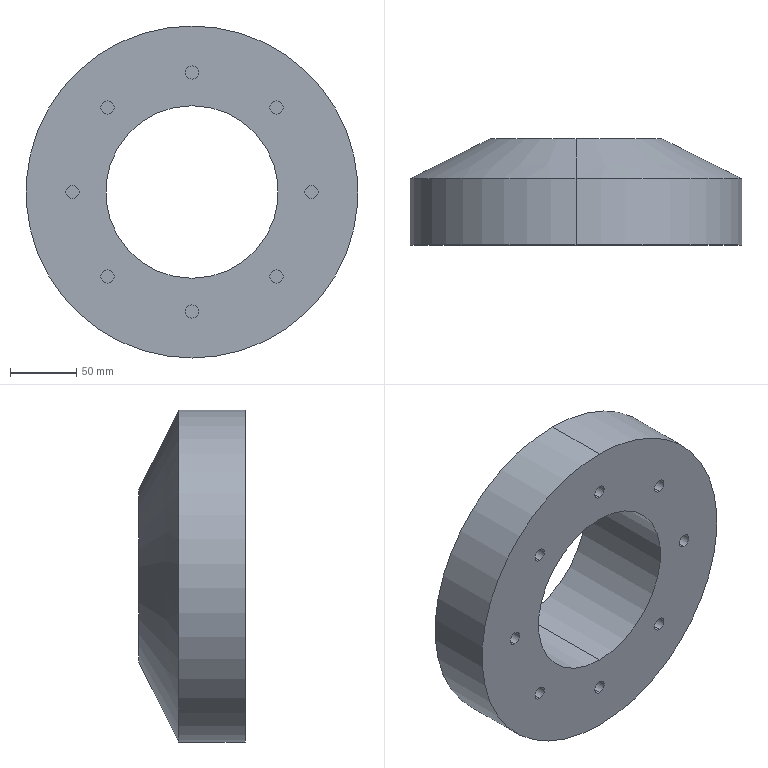Part | SolidWorks | features ICE 1, Revolution 1 | 1 solid | 31 faces | box 250 x 80 x 250 mm | volume 2252522 mm3 | cylinder 20 | plane 9 | cone 2 | commonest cylinder face diameters 10 x16 130 x2 250 x2
STEP:
#1=CARTESIAN_POINT('',(63.64,-23.992,-58.64));
#2=VERTEX_POINT('',#1);
#3=CARTESIAN_POINT('',(63.64,-23.992,-68.64));
#4=VERTEX_POINT('',#3);
#5=CARTESIAN_POINT('',(63.64,-23.992,-63.64));
#6=DIRECTION('',(0.,-1.,0.));
#7=DIRECTION('',(0.,0.,-1.));
#8=AXIS2_PLACEMENT_3D('',#5,#6,#7);
#9=CIRCLE('',#8,5.);
#10=EDGE_CURVE('',#2,#4,#9,.T.);
#11=ORIENTED_EDGE('',*,*,#10,.F.);
#12=CARTESIAN_POINT('',(63.64,-53.992,-58.64));
#13=VERTEX_POINT('',#12);
#14=CARTESIAN_POINT('',(63.64,-23.992,-58.64));
#15=DIRECTION('',(0.,-1.,0.));
#16=VECTOR('',#15,1000.);
#17=LINE('',#14,#16);
#18=EDGE_CURVE('',#2,#13,#17,.T.);
#19=ORIENTED_EDGE('',*,*,#18,.T.);
#20=CARTESIAN_POINT('',(63.64,-53.992,-68.64));
#21=VERTEX_POINT('',#20);
#22=CARTESIAN_POINT('',(63.64,-53.992,-63.64));
#23=DIRECTION('',(0.,-1.,0.));
#24=DIRECTION('',(0.,0.,-1.));
#25=AXIS2_PLACEMENT_3D('',#22,#23,#24);
#26=CIRCLE('',#25,5.);
#27=EDGE_CURVE('',#13,#21,#26,.T.);
#28=ORIENTED_EDGE('',*,*,#27,.T.);
#29=CARTESIAN_POINT('',(63.64,-23.992,-68.64));
#30=DIRECTION('',(0.,-1.,0.));
#31=VECTOR('',#30,1000.);
#32=LINE('',#29,#31);
#33=EDGE_CURVE('',#4,#21,#32,.T.);
#34=ORIENTED_EDGE('',*,*,#33,.F.);
#35=EDGE_LOOP('',(#11,#19,#28,#34));
#36=FACE_OUTER_BOUND('',#35,.T.);
#37=CARTESIAN_POINT('',(63.64,-23.992,-63.64));
#38=DIRECTION('',(0.,-1.,0.));
#39=DIRECTION('',(0.,0.,-1.));
#40=AXIS2_PLACEMENT_3D('',#37,#38,#39);
#41=CYLINDRICAL_SURFACE('',#40,5.);
#42=ADVANCED_FACE('',(#36),#41,.F.);
#43=CARTESIAN_POINT('',(0.,-23.992,-85.));
#44=VERTEX_POINT('',#43);
#45=CARTESIAN_POINT('',(0.,-23.992,-95.));
#46=VERTEX_POINT('',#45);
#47=CARTESIAN_POINT('',(0.,-23.992,-90.));
#48=DIRECTION('',(0.,-1.,0.));
#49=DIRECTION('',(0.,0.,-1.));
#50=AXIS2_PLACEMENT_3D('',#47,#48,#49);
#51=CIRCLE('',#50,5.);
#52=EDGE_CURVE('',#44,#46,#51,.T.);
#53=ORIENTED_EDGE('',*,*,#52,.F.);
#54=CARTESIAN_POINT('',(0.,-53.992,-85.));
#55=VERTEX_POINT('',#54);
#56=CARTESIAN_POINT('',(0.,-23.992,-85.));
#57=DIRECTION('',(0.,-1.,0.));
#58=VECTOR('',#57,1000.);
#59=LINE('',#56,#58);
#60=EDGE_CURVE('',#44,#55,#59,.T.);
#61=ORIENTED_EDGE('',*,*,#60,.T.);
#62=CARTESIAN_POINT('',(0.,-53.992,-95.));
#63=VERTEX_POINT('',#62);
#64=CARTESIAN_POINT('',(0.,-53.992,-90.));
#65=DIRECTION('',(0.,-1.,0.));
#66=DIRECTION('',(0.,0.,-1.));
#67=AXIS2_PLACEMENT_3D('',#64,#65,#66);
#68=CIRCLE('',#67,5.);
#69=EDGE_CURVE('',#55,#63,#68,.T.);
#70=ORIENTED_EDGE('',*,*,#69,.T.);
#71=CARTESIAN_POINT('',(0.,-23.992,-95.));
#72=DIRECTION('',(0.,-1.,0.));
#73=VECTOR('',#72,1000.);
#74=LINE('',#71,#73);
#75=EDGE_CURVE('',#46,#63,#74,.T.);
#76=ORIENTED_EDGE('',*,*,#75,.F.);
#77=EDGE_LOOP('',(#53,#61,#70,#76));
#78=FACE_OUTER_BOUND('',#77,.T.);
#79=CARTESIAN_POINT('',(0.,-23.992,-90.));
#80=DIRECTION('',(0.,-1.,0.));
#81=DIRECTION('',(0.,0.,-1.));
#82=AXIS2_PLACEMENT_3D('',#79,#80,#81);
#83=CYLINDRICAL_SURFACE('',#82,5.);
#84=ADVANCED_FACE('',(#78),#83,.F.);
#85=CARTESIAN_POINT('',(-63.64,-23.992,-58.64));
#86=VERTEX_POINT('',#85);
#87=CARTESIAN_POINT('',(-63.64,-23.992,-68.64));
#88=VERTEX_POINT('',#87);
#89=CARTESIAN_POINT('',(-63.64,-23.992,-63.64));
#90=DIRECTION('',(0.,-1.,0.));
#91=DIRECTION('',(0.,0.,-1.));
#92=AXIS2_PLACEMENT_3D('',#89,#90,#91);
#93=CIRCLE('',#92,5.);
#94=EDGE_CURVE('',#86,#88,#93,.T.);
#95=ORIENTED_EDGE('',*,*,#94,.F.);
#96=CARTESIAN_POINT('',(-63.64,-53.992,-58.64));
#97=VERTEX_POINT('',#96);
#98=CARTESIAN_POINT('',(-63.64,-23.992,-58.64));
#99=DIRECTION('',(0.,-1.,0.));
#100=VECTOR('',#99,1000.);
#101=LINE('',#98,#100);
#102=EDGE_CURVE('',#86,#97,#101,.T.);
#103=ORIENTED_EDGE('',*,*,#102,.T.);
#104=CARTESIAN_POINT('',(-63.64,-53.992,-68.64));
#105=VERTEX_POINT('',#104);
#106=CARTESIAN_POINT('',(-63.64,-53.992,-63.64));
#107=DIRECTION('',(0.,-1.,0.));
#108=DIRECTION('',(0.,0.,-1.));
#109=AXIS2_PLACEMENT_3D('',#106,#107,#108);
#110=CIRCLE('',#109,5.);
#111=EDGE_CURVE('',#97,#105,#110,.T.);
#112=ORIENTED_EDGE('',*,*,#111,.T.);
#113=CARTESIAN_POINT('',(-63.64,-23.992,-68.64));
#114=DIRECTION('',(0.,-1.,0.));
#115=VECTOR('',#114,1000.);
#116=LINE('',#113,#115);
#117=EDGE_CURVE('',#88,#105,#116,.T.);
#118=ORIENTED_EDGE('',*,*,#117,.F.);
#119=EDGE_LOOP('',(#95,#103,#112,#118));
#120=FACE_OUTER_BOUND('',#119,.T.);
#121=CARTESIAN_POINT('',(-63.64,-23.992,-63.64));
#122=DIRECTION('',(0.,-1.,0.));
#123=DIRECTION('',(0.,0.,-1.));
#124=AXIS2_PLACEMENT_3D('',#121,#122,#123);
#125=CYLINDRICAL_SURFACE('',#124,5.);
#126=ADVANCED_FACE('',(#120),#125,.F.);
#127=CARTESIAN_POINT('',(-90.,-23.992,5.));
#128=VERTEX_POINT('',#127);
#129=CARTESIAN_POINT('',(-90.,-23.992,-5.));
#130=VERTEX_POINT('',#129);
#131=CARTESIAN_POINT('',(-90.,-23.992,0.));
#132=DIRECTION('',(0.,-1.,0.));
#133=DIRECTION('',(0.,0.,-1.));
#134=AXIS2_PLACEMENT_3D('',#131,#132,#133);
#135=CIRCLE('',#134,5.);
#136=EDGE_CURVE('',#128,#130,#135,.T.);
#137=ORIENTED_EDGE('',*,*,#136,.F.);
#138=CARTESIAN_POINT('',(-90.,-53.992,5.));
#139=VERTEX_POINT('',#138);
#140=CARTESIAN_POINT('',(-90.,-23.992,5.));
#141=DIRECTION('',(0.,-1.,0.));
#142=VECTOR('',#141,1000.);
#143=LINE('',#140,#142);
#144=EDGE_CURVE('',#128,#139,#143,.T.);
#145=ORIENTED_EDGE('',*,*,#144,.T.);
#146=CARTESIAN_POINT('',(-90.,-53.992,-5.));
#147=VERTEX_POINT('',#146);
#148=CARTESIAN_POINT('',(-90.,-53.992,0.));
#149=DIRECTION('',(0.,-1.,0.));
#150=DIRECTION('',(0.,0.,-1.));
#151=AXIS2_PLACEMENT_3D('',#148,#149,#150);
#152=CIRCLE('',#151,5.);
#153=EDGE_CURVE('',#139,#147,#152,.T.);
#154=ORIENTED_EDGE('',*,*,#153,.T.);
#155=CARTESIAN_POINT('',(-90.,-23.992,-5.));
#156=DIRECTION('',(0.,-1.,0.));
#157=VECTOR('',#156,1000.);
#158=LINE('',#155,#157);
#159=EDGE_CURVE('',#130,#147,#158,.T.);
#160=ORIENTED_EDGE('',*,*,#159,.F.);
#161=EDGE_LOOP('',(#137,#145,#154,#160));
#162=FACE_OUTER_BOUND('',#161,.T.);
#163=CARTESIAN_POINT('',(-90.,-23.992,0.));
#164=DIRECTION('',(0.,-1.,0.));
#165=DIRECTION('',(0.,0.,-1.));
#166=AXIS2_PLACEMENT_3D('',#163,#164,#165);
#167=CYLINDRICAL_SURFACE('',#166,5.);
#168=ADVANCED_FACE('',(#162),#167,.F.);
#169=CARTESIAN_POINT('',(-63.64,-23.992,68.64));
#170=VERTEX_POINT('',#169);
#171=CARTESIAN_POINT('',(-63.64,-23.992,58.64));
#172=VERTEX_POINT('',#171);
#173=CARTESIAN_POINT('',(-63.64,-23.992,63.64));
#174=DIRECTION('',(0.,-1.,0.));
#175=DIRECTION('',(0.,0.,-1.));
#176=AXIS2_PLACEMENT_3D('',#173,#174,#175);
#177=CIRCLE('',#176,5.);
#178=EDGE_CURVE('',#170,#172,#177,.T.);
#179=ORIENTED_EDGE('',*,*,#178,.F.);
#180=CARTESIAN_POINT('',(-63.64,-53.992,68.64));
#181=VERTEX_POINT('',#180);
#182=CARTESIAN_POINT('',(-63.64,-23.992,68.64));
#183=DIRECTION('',(0.,-1.,0.));
#184=VECTOR('',#183,1000.);
#185=LINE('',#182,#184);
#186=EDGE_CURVE('',#170,#181,#185,.T.);
#187=ORIENTED_EDGE('',*,*,#186,.T.);
#188=CARTESIAN_POINT('',(-63.64,-53.992,58.64));
#189=VERTEX_POINT('',#188);
#190=CARTESIAN_POINT('',(-63.64,-53.992,63.64));
#191=DIRECTION('',(0.,-1.,0.));
#192=DIRECTION('',(0.,0.,-1.));
#193=AXIS2_PLACEMENT_3D('',#190,#191,#192);
#194=CIRCLE('',#193,5.);
#195=EDGE_CURVE('',#181,#189,#194,.T.);
#196=ORIENTED_EDGE('',*,*,#195,.T.);
#197=CARTESIAN_POINT('',(-63.64,-23.992,58.64));
#198=DIRECTION('',(0.,-1.,0.));
#199=VECTOR('',#198,1000.);
#200=LINE('',#197,#199);
#201=EDGE_CURVE('',#172,#189,#200,.T.);
#202=ORIENTED_EDGE('',*,*,#201,.F.);
#203=EDGE_LOOP('',(#179,#187,#196,#202));
#204=FACE_OUTER_BOUND('',#203,.T.);
#205=CARTESIAN_POINT('',(-63.64,-23.992,63.64));
#206=DIRECTION('',(0.,-1.,0.));
#207=DIRECTION('',(0.,0.,-1.));
#208=AXIS2_PLACEMENT_3D('',#205,#206,#207);
#209=CYLINDRICAL_SURFACE('',#208,5.);
#210=ADVANCED_FACE('',(#204),#209,.F.);
#211=CARTESIAN_POINT('',(0.,-23.992,95.));
#212=VERTEX_POINT('',#211);
#213=CARTESIAN_POINT('',(0.,-23.992,85.));
#214=VERTEX_POINT('',#213);
#215=CARTESIAN_POINT('',(0.,-23.992,90.));
#216=DIRECTION('',(0.,-1.,0.));
#217=DIRECTION('',(0.,0.,-1.));
#218=AXIS2_PLACEMENT_3D('',#215,#216,#217);
#219=CIRCLE('',#218,5.);
#220=EDGE_CURVE('',#212,#214,#219,.T.);
#221=ORIENTED_EDGE('',*,*,#220,.F.);
#222=CARTESIAN_POINT('',(0.,-53.992,95.));
#223=VERTEX_POINT('',#222);
#224=CARTESIAN_POINT('',(0.,-23.992,95.));
#225=DIRECTION('',(0.,-1.,0.));
#226=VECTOR('',#225,1000.);
#227=LINE('',#224,#226);
#228=EDGE_CURVE('',#212,#223,#227,.T.);
#229=ORIENTED_EDGE('',*,*,#228,.T.);
#230=CARTESIAN_POINT('',(0.,-53.992,85.));
#231=VERTEX_POINT('',#230);
#232=CARTESIAN_POINT('',(0.,-53.992,90.));
#233=DIRECTION('',(0.,-1.,0.));
#234=DIRECTION('',(0.,0.,-1.));
#235=AXIS2_PLACEMENT_3D('',#232,#233,#234);
#236=CIRCLE('',#235,5.);
#237=EDGE_CURVE('',#223,#231,#236,.T.);
#238=ORIENTED_EDGE('',*,*,#237,.T.);
#239=CARTESIAN_POINT('',(0.,-23.992,85.));
#240=DIRECTION('',(0.,-1.,0.));
#241=VECTOR('',#240,1000.);
#242=LINE('',#239,#241);
#243=EDGE_CURVE('',#214,#231,#242,.T.);
#244=ORIENTED_EDGE('',*,*,#243,.F.);
#245=EDGE_LOOP('',(#221,#229,#238,#244));
#246=FACE_OUTER_BOUND('',#245,.T.);
#247=CARTESIAN_POINT('',(0.,-23.992,90.));
#248=DIRECTION('',(0.,-1.,0.));
#249=DIRECTION('',(0.,0.,-1.));
#250=AXIS2_PLACEMENT_3D('',#247,#248,#249);
#251=CYLINDRICAL_SURFACE('',#250,5.);
#252=ADVANCED_FACE('',(#246),#251,.F.);
#253=CARTESIAN_POINT('',(63.64,-23.992,68.64));
#254=VERTEX_POINT('',#253);
#255=CARTESIAN_POINT('',(63.64,-23.992,58.64));
#256=VERTEX_POINT('',#255);
#257=CARTESIAN_POINT('',(63.64,-23.992,63.64));
#258=DIRECTION('',(0.,-1.,0.));
#259=DIRECTION('',(0.,0.,-1.));
#260=AXIS2_PLACEMENT_3D('',#257,#258,#259);
#261=CIRCLE('',#260,5.);
#262=EDGE_CURVE('',#254,#256,#261,.T.);
#263=ORIENTED_EDGE('',*,*,#262,.F.);
#264=CARTESIAN_POINT('',(63.64,-53.992,68.64));
#265=VERTEX_POINT('',#264);
#266=CARTESIAN_POINT('',(63.64,-23.992,68.64));
#267=DIRECTION('',(0.,-1.,0.));
#268=VECTOR('',#267,1000.);
#269=LINE('',#266,#268);
#270=EDGE_CURVE('',#254,#265,#269,.T.);
#271=ORIENTED_EDGE('',*,*,#270,.T.);
#272=CARTESIAN_POINT('',(63.64,-53.992,58.64));
#273=VERTEX_POINT('',#272);
#274=CARTESIAN_POINT('',(63.64,-53.992,63.64));
#275=DIRECTION('',(0.,-1.,0.));
#276=DIRECTION('',(0.,0.,-1.));
#277=AXIS2_PLACEMENT_3D('',#274,#275,#276);
#278=CIRCLE('',#277,5.);
#279=EDGE_CURVE('',#265,#273,#278,.T.);
#280=ORIENTED_EDGE('',*,*,#279,.T.);
#281=CARTESIAN_POINT('',(63.64,-23.992,58.64));
#282=DIRECTION('',(0.,-1.,0.));
#283=VECTOR('',#282,1000.);
#284=LINE('',#281,#283);
#285=EDGE_CURVE('',#256,#273,#284,.T.);
#286=ORIENTED_EDGE('',*,*,#285,.F.);
#287=EDGE_LOOP('',(#263,#271,#280,#286));
#288=FACE_OUTER_BOUND('',#287,.T.);
#289=CARTESIAN_POINT('',(63.64,-23.992,63.64));
#290=DIRECTION('',(0.,-1.,0.));
#291=DIRECTION('',(0.,0.,-1.));
#292=AXIS2_PLACEMENT_3D('',#289,#290,#291);
#293=CYLINDRICAL_SURFACE('',#292,5.);
#294=ADVANCED_FACE('',(#288),#293,.F.);
#295=CARTESIAN_POINT('',(90.,-23.992,5.));
#296=VERTEX_POINT('',#295);
#297=CARTESIAN_POINT('',(90.,-23.992,-5.));
#298=VERTEX_POINT('',#297);
#299=CARTESIAN_POINT('',(90.,-23.992,0.));
#300=DIRECTION('',(0.,-1.,0.));
#301=DIRECTION('',(0.,0.,-1.));
#302=AXIS2_PLACEMENT_3D('',#299,#300,#301);
#303=CIRCLE('',#302,5.);
#304=EDGE_CURVE('',#296,#298,#303,.T.);
#305=ORIENTED_EDGE('',*,*,#304,.F.);
#306=CARTESIAN_POINT('',(90.,-53.992,5.));
#307=VERTEX_POINT('',#306);
#308=CARTESIAN_POINT('',(90.,-23.992,5.));
#309=DIRECTION('',(0.,-1.,0.));
#310=VECTOR('',#309,1000.);
#311=LINE('',#308,#310);
#312=EDGE_CURVE('',#296,#307,#311,.T.);
#313=ORIENTED_EDGE('',*,*,#312,.T.);
#314=CARTESIAN_POINT('',(90.,-53.992,-5.));
#315=VERTEX_POINT('',#314);
#316=CARTESIAN_POINT('',(90.,-53.992,0.));
#317=DIRECTION('',(0.,-1.,0.));
#318=DIRECTION('',(0.,0.,-1.));
#319=AXIS2_PLACEMENT_3D('',#316,#317,#318);
#320=CIRCLE('',#319,5.);
#321=EDGE_CURVE('',#307,#315,#320,.T.);
#322=ORIENTED_EDGE('',*,*,#321,.T.);
#323=CARTESIAN_POINT('',(90.,-23.992,-5.));
#324=DIRECTION('',(0.,-1.,0.));
#325=VECTOR('',#324,1000.);
#326=LINE('',#323,#325);
#327=EDGE_CURVE('',#298,#315,#326,.T.);
#328=ORIENTED_EDGE('',*,*,#327,.F.);
#329=EDGE_LOOP('',(#305,#313,#322,#328));
#330=FACE_OUTER_BOUND('',#329,.T.);
#331=CARTESIAN_POINT('',(90.,-23.992,0.));
#332=DIRECTION('',(0.,-1.,0.));
#333=DIRECTION('',(0.,0.,-1.));
#334=AXIS2_PLACEMENT_3D('',#331,#332,#333);
#335=CYLINDRICAL_SURFACE('',#334,5.);
#336=ADVANCED_FACE('',(#330),#335,.F.);
#337=CARTESIAN_POINT('',(0.,-53.992,125.));
#338=VERTEX_POINT('',#337);
#339=CARTESIAN_POINT('',(0.,-53.992,-125.));
#340=VERTEX_POINT('',#339);
#341=CARTESIAN_POINT('',(0.,-53.992,0.));
#342=DIRECTION('',(0.,1.,0.));
#343=DIRECTION('',(0.,0.,1.));
#344=AXIS2_PLACEMENT_3D('',#341,#342,#343);
#345=CIRCLE('',#344,125.);
#346=EDGE_CURVE('',#338,#340,#345,.T.);
#347=ORIENTED_EDGE('',*,*,#346,.T.);
#348=CARTESIAN_POINT('',(0.,-3.992,-125.));
#349=VERTEX_POINT('',#348);
#350=CARTESIAN_POINT('',(0.,116.895,-125.));
#351=DIRECTION('',(0.,1.,0.));
#352=VECTOR('',#351,1000.);
#353=LINE('',#350,#352);
#354=EDGE_CURVE('',#340,#349,#353,.T.);
#355=ORIENTED_EDGE('',*,*,#354,.T.);
#356=CARTESIAN_POINT('',(0.,-3.992,125.));
#357=VERTEX_POINT('',#356);
#358=CARTESIAN_POINT('',(0.,-3.992,0.));
#359=DIRECTION('',(0.,1.,0.));
#360=DIRECTION('',(0.,0.,1.));
#361=AXIS2_PLACEMENT_3D('',#358,#359,#360);
#362=CIRCLE('',#361,125.);
#363=EDGE_CURVE('',#357,#349,#362,.T.);
#364=ORIENTED_EDGE('',*,*,#363,.F.);
#365=CARTESIAN_POINT('',(0.,116.895,125.));
#366=DIRECTION('',(0.,1.,0.));
#367=VECTOR('',#366,1000.);
#368=LINE('',#365,#367);
#369=EDGE_CURVE('',#338,#357,#368,.T.);
#370=ORIENTED_EDGE('',*,*,#369,.F.);
#371=EDGE_LOOP('',(#347,#355,#364,#370));
#372=FACE_OUTER_BOUND('',#371,.T.);
#373=CARTESIAN_POINT('',(0.,116.895,0.));
#374=DIRECTION('',(0.,1.,0.));
#375=DIRECTION('',(0.,0.,1.));
#376=AXIS2_PLACEMENT_3D('',#373,#374,#375);
#377=CYLINDRICAL_SURFACE('',#376,125.);
#378=ADVANCED_FACE('',(#372),#377,.T.);
#379=CARTESIAN_POINT('',(0.,26.008,65.));
#380=VERTEX_POINT('',#379);
#381=CARTESIAN_POINT('',(0.,26.008,-65.));
#382=VERTEX_POINT('',#381);
#383=CARTESIAN_POINT('',(0.,26.008,0.));
#384=DIRECTION('',(0.,1.,0.));
#385=DIRECTION('',(0.,0.,1.));
#386=AXIS2_PLACEMENT_3D('',#383,#384,#385);
#387=CIRCLE('',#386,65.);
#388=EDGE_CURVE('',#380,#382,#387,.T.);
#389=ORIENTED_EDGE('',*,*,#388,.F.);
#390=CARTESIAN_POINT('',(0.,-3.992,125.));
#391=DIRECTION('',(0.,-0.4472,0.8944));
#392=VECTOR('',#391,1000.);
#393=LINE('',#390,#392);
#394=EDGE_CURVE('',#380,#357,#393,.T.);
#395=ORIENTED_EDGE('',*,*,#394,.T.);
#396=ORIENTED_EDGE('',*,*,#363,.T.);
#397=CARTESIAN_POINT('',(0.,-3.992,-125.));
#398=DIRECTION('',(0.,-0.4472,-0.8944));
#399=VECTOR('',#398,1000.);
#400=LINE('',#397,#399);
#401=EDGE_CURVE('',#382,#349,#400,.T.);
#402=ORIENTED_EDGE('',*,*,#401,.F.);
#403=EDGE_LOOP('',(#389,#395,#396,#402));
#404=FACE_OUTER_BOUND('',#403,.T.);
#405=CARTESIAN_POINT('',(0.,-3.992,0.));
#406=DIRECTION('',(0.,-1.,0.));
#407=DIRECTION('',(0.,0.,-1.));
#408=AXIS2_PLACEMENT_3D('',#405,#406,#407);
#409=CONICAL_SURFACE('',#408,125.,1.107);
#410=ADVANCED_FACE('',(#404),#409,.T.);
#411=CARTESIAN_POINT('',(0.,-53.992,-65.));
#412=VERTEX_POINT('',#411);
#413=CARTESIAN_POINT('',(0.,-53.992,65.));
#414=VERTEX_POINT('',#413);
#415=CARTESIAN_POINT('',(0.,-53.992,0.));
#416=DIRECTION('',(0.,1.,0.));
#417=DIRECTION('',(0.,0.,1.));
#418=AXIS2_PLACEMENT_3D('',#415,#416,#417);
#419=CIRCLE('',#418,65.);
#420=EDGE_CURVE('',#412,#414,#419,.T.);
#421=ORIENTED_EDGE('',*,*,#420,.F.);
#422=CARTESIAN_POINT('',(0.,116.895,-65.));
#423=DIRECTION('',(0.,1.,0.));
#424=VECTOR('',#423,1000.);
#425=LINE('',#422,#424);
#426=EDGE_CURVE('',#412,#382,#425,.T.);
#427=ORIENTED_EDGE('',*,*,#426,.T.);
#428=CARTESIAN_POINT('',(0.,26.008,0.));
#429=DIRECTION('',(0.,1.,0.));
#430=DIRECTION('',(0.,0.,1.));
#431=AXIS2_PLACEMENT_3D('',#428,#429,#430);
#432=CIRCLE('',#431,65.);
#433=EDGE_CURVE('',#382,#380,#432,.T.);
#434=ORIENTED_EDGE('',*,*,#433,.T.);
#435=CARTESIAN_POINT('',(0.,116.895,65.));
#436=DIRECTION('',(0.,1.,0.));
#437=VECTOR('',#436,1000.);
#438=LINE('',#435,#437);
#439=EDGE_CURVE('',#414,#380,#438,.T.);
#440=ORIENTED_EDGE('',*,*,#439,.F.);
#441=EDGE_LOOP('',(#421,#427,#434,#440));
#442=FACE_OUTER_BOUND('',#441,.T.);
#443=CARTESIAN_POINT('',(0.,116.895,0.));
#444=DIRECTION('',(0.,1.,0.));
#445=DIRECTION('',(0.,0.,1.));
#446=AXIS2_PLACEMENT_3D('',#443,#444,#445);
#447=CYLINDRICAL_SURFACE('',#446,65.);
#448=ADVANCED_FACE('',(#442),#447,.F.);
#449=CARTESIAN_POINT('',(63.64,-53.992,-63.64));
#450=DIRECTION('',(0.,-1.,0.));
#451=DIRECTION('',(0.,0.,-1.));
#452=AXIS2_PLACEMENT_3D('',#449,#450,#451);
#453=CIRCLE('',#452,5.);
#454=EDGE_CURVE('',#21,#13,#453,.T.);
#455=ORIENTED_EDGE('',*,*,#454,.F.);
#456=ORIENTED_EDGE('',*,*,#27,.F.);
#457=EDGE_LOOP('',(#455,#456));
#458=FACE_BOUND('',#457,.T.);
#459=CARTESIAN_POINT('',(0.,-53.992,-90.));
#460=DIRECTION('',(0.,-1.,0.));
#461=DIRECTION('',(0.,0.,-1.));
#462=AXIS2_PLACEMENT_3D('',#459,#460,#461);
#463=CIRCLE('',#462,5.);
#464=EDGE_CURVE('',#63,#55,#463,.T.);
#465=ORIENTED_EDGE('',*,*,#464,.F.);
#466=ORIENTED_EDGE('',*,*,#69,.F.);
#467=EDGE_LOOP('',(#465,#466));
#468=FACE_BOUND('',#467,.T.);
#469=CARTESIAN_POINT('',(-63.64,-53.992,-63.64));
#470=DIRECTION('',(0.,-1.,0.));
#471=DIRECTION('',(0.,0.,-1.));
#472=AXIS2_PLACEMENT_3D('',#469,#470,#471);
#473=CIRCLE('',#472,5.);
#474=EDGE_CURVE('',#105,#97,#473,.T.);
#475=ORIENTED_EDGE('',*,*,#474,.F.);
#476=ORIENTED_EDGE('',*,*,#111,.F.);
#477=EDGE_LOOP('',(#475,#476));
#478=FACE_BOUND('',#477,.T.);
#479=CARTESIAN_POINT('',(-90.,-53.992,0.));
#480=DIRECTION('',(0.,-1.,0.));
#481=DIRECTION('',(0.,0.,-1.));
#482=AXIS2_PLACEMENT_3D('',#479,#480,#481);
#483=CIRCLE('',#482,5.);
#484=EDGE_CURVE('',#147,#139,#483,.T.);
#485=ORIENTED_EDGE('',*,*,#484,.F.);
#486=ORIENTED_EDGE('',*,*,#153,.F.);
#487=EDGE_LOOP('',(#485,#486));
#488=FACE_BOUND('',#487,.T.);
#489=CARTESIAN_POINT('',(-63.64,-53.992,63.64));
#490=DIRECTION('',(0.,-1.,0.));
#491=DIRECTION('',(0.,0.,-1.));
#492=AXIS2_PLACEMENT_3D('',#489,#490,#491);
#493=CIRCLE('',#492,5.);
#494=EDGE_CURVE('',#189,#181,#493,.T.);
#495=ORIENTED_EDGE('',*,*,#494,.F.);
#496=ORIENTED_EDGE('',*,*,#195,.F.);
#497=EDGE_LOOP('',(#495,#496));
#498=FACE_BOUND('',#497,.T.);
#499=CARTESIAN_POINT('',(0.,-53.992,90.));
#500=DIRECTION('',(0.,-1.,0.));
#501=DIRECTION('',(0.,0.,-1.));
#502=AXIS2_PLACEMENT_3D('',#499,#500,#501);
#503=CIRCLE('',#502,5.);
#504=EDGE_CURVE('',#231,#223,#503,.T.);
#505=ORIENTED_EDGE('',*,*,#504,.F.);
#506=ORIENTED_EDGE('',*,*,#237,.F.);
#507=EDGE_LOOP('',(#505,#506));
#508=FACE_BOUND('',#507,.T.);
#509=CARTESIAN_POINT('',(63.64,-53.992,63.64));
#510=DIRECTION('',(0.,-1.,0.));
#511=DIRECTION('',(0.,0.,-1.));
#512=AXIS2_PLACEMENT_3D('',#509,#510,#511);
#513=CIRCLE('',#512,5.);
#514=EDGE_CURVE('',#273,#265,#513,.T.);
#515=ORIENTED_EDGE('',*,*,#514,.F.);
#516=ORIENTED_EDGE('',*,*,#279,.F.);
#517=EDGE_LOOP('',(#515,#516));
#518=FACE_BOUND('',#517,.T.);
#519=CARTESIAN_POINT('',(90.,-53.992,0.));
#520=DIRECTION('',(0.,-1.,0.));
#521=DIRECTION('',(0.,0.,-1.));
#522=AXIS2_PLACEMENT_3D('',#519,#520,#521);
#523=CIRCLE('',#522,5.);
#524=EDGE_CURVE('',#315,#307,#523,.T.);
#525=ORIENTED_EDGE('',*,*,#524,.F.);
#526=ORIENTED_EDGE('',*,*,#321,.F.);
#527=EDGE_LOOP('',(#525,#526));
#528=FACE_BOUND('',#527,.T.);
#529=ORIENTED_EDGE('',*,*,#346,.F.);
#530=CARTESIAN_POINT('',(0.,-53.992,0.));
#531=DIRECTION('',(0.,1.,0.));
#532=DIRECTION('',(0.,0.,1.));
#533=AXIS2_PLACEMENT_3D('',#530,#531,#532);
#534=CIRCLE('',#533,125.);
#535=EDGE_CURVE('',#340,#338,#534,.T.);
#536=ORIENTED_EDGE('',*,*,#535,.F.);
#537=EDGE_LOOP('',(#529,#536));
#538=FACE_OUTER_BOUND('',#537,.T.);
#539=CARTESIAN_POINT('',(0.,-53.992,0.));
#540=DIRECTION('',(0.,1.,0.));
#541=DIRECTION('',(0.,0.,1.));
#542=AXIS2_PLACEMENT_3D('',#539,#540,#541);
#543=CIRCLE('',#542,65.);
#544=EDGE_CURVE('',#414,#412,#543,.T.);
#545=ORIENTED_EDGE('',*,*,#544,.T.);
#546=ORIENTED_EDGE('',*,*,#420,.T.);
#547=EDGE_LOOP('',(#545,#546));
#548=FACE_BOUND('',#547,.T.);
#549=CARTESIAN_POINT('',(125.,-53.992,0.));
#550=DIRECTION('',(0.,1.,0.));
#551=DIRECTION('',(0.,0.,1.));
#552=AXIS2_PLACEMENT_3D('',#549,#550,#551);
#553=PLANE('',#552);
#554=ADVANCED_FACE('',(#458,#468,#478,#488,#498,#508,#518,#528,#538,#548),#553,.F.);
#555=ORIENTED_EDGE('',*,*,#426,.F.);
#556=ORIENTED_EDGE('',*,*,#544,.F.);
#557=ORIENTED_EDGE('',*,*,#439,.T.);
#558=ORIENTED_EDGE('',*,*,#388,.T.);
#559=EDGE_LOOP('',(#555,#556,#557,#558));
#560=FACE_OUTER_BOUND('',#559,.T.);
#561=CARTESIAN_POINT('',(0.,116.895,0.));
#562=DIRECTION('',(0.,1.,0.));
#563=DIRECTION('',(0.,0.,1.));
#564=AXIS2_PLACEMENT_3D('',#561,#562,#563);
#565=CYLINDRICAL_SURFACE('',#564,65.);
#566=ADVANCED_FACE('',(#560),#565,.F.);
#567=ORIENTED_EDGE('',*,*,#394,.F.);
#568=ORIENTED_EDGE('',*,*,#433,.F.);
#569=ORIENTED_EDGE('',*,*,#401,.T.);
#570=CARTESIAN_POINT('',(0.,-3.992,0.));
#571=DIRECTION('',(0.,1.,0.));
#572=DIRECTION('',(0.,0.,1.));
#573=AXIS2_PLACEMENT_3D('',#570,#571,#572);
#574=CIRCLE('',#573,125.);
#575=EDGE_CURVE('',#349,#357,#574,.T.);
#576=ORIENTED_EDGE('',*,*,#575,.T.);
#577=EDGE_LOOP('',(#567,#568,#569,#576));
#578=FACE_OUTER_BOUND('',#577,.T.);
#579=CARTESIAN_POINT('',(0.,-3.992,0.));
#580=DIRECTION('',(0.,-1.,0.));
#581=DIRECTION('',(0.,0.,-1.));
#582=AXIS2_PLACEMENT_3D('',#579,#580,#581);
#583=CONICAL_SURFACE('',#582,125.,1.107);
#584=ADVANCED_FACE('',(#578),#583,.T.);
#585=ORIENTED_EDGE('',*,*,#354,.F.);
#586=ORIENTED_EDGE('',*,*,#535,.T.);
#587=ORIENTED_EDGE('',*,*,#369,.T.);
#588=ORIENTED_EDGE('',*,*,#575,.F.);
#589=EDGE_LOOP('',(#585,#586,#587,#588));
#590=FACE_OUTER_BOUND('',#589,.T.);
#591=CARTESIAN_POINT('',(0.,116.895,0.));
#592=DIRECTION('',(0.,1.,0.));
#593=DIRECTION('',(0.,0.,1.));
#594=AXIS2_PLACEMENT_3D('',#591,#592,#593);
#595=CYLINDRICAL_SURFACE('',#594,125.);
#596=ADVANCED_FACE('',(#590),#595,.T.);
#597=ORIENTED_EDGE('',*,*,#312,.F.);
#598=CARTESIAN_POINT('',(90.,-23.992,0.));
#599=DIRECTION('',(0.,-1.,0.));
#600=DIRECTION('',(0.,0.,-1.));
#601=AXIS2_PLACEMENT_3D('',#598,#599,#600);
#602=CIRCLE('',#601,5.);
#603=EDGE_CURVE('',#298,#296,#602,.T.);
#604=ORIENTED_EDGE('',*,*,#603,.F.);
#605=ORIENTED_EDGE('',*,*,#327,.T.);
#606=ORIENTED_EDGE('',*,*,#524,.T.);
#607=EDGE_LOOP('',(#597,#604,#605,#606));
#608=FACE_OUTER_BOUND('',#607,.T.);
#609=CARTESIAN_POINT('',(90.,-23.992,0.));
#610=DIRECTION('',(0.,-1.,0.));
#611=DIRECTION('',(0.,0.,-1.));
#612=AXIS2_PLACEMENT_3D('',#609,#610,#611);
#613=CYLINDRICAL_SURFACE('',#612,5.);
#614=ADVANCED_FACE('',(#608),#613,.F.);
#615=ORIENTED_EDGE('',*,*,#603,.T.);
#616=ORIENTED_EDGE('',*,*,#304,.T.);
#617=EDGE_LOOP('',(#615,#616));
#618=FACE_OUTER_BOUND('',#617,.T.);
#619=CARTESIAN_POINT('',(90.,-23.992,0.));
#620=DIRECTION('',(0.,-1.,0.));
#621=DIRECTION('',(0.,0.,-1.));
#622=AXIS2_PLACEMENT_3D('',#619,#620,#621);
#623=PLANE('',#622);
#624=ADVANCED_FACE('',(#618),#623,.T.);
#625=ORIENTED_EDGE('',*,*,#270,.F.);
#626=CARTESIAN_POINT('',(63.64,-23.992,63.64));
#627=DIRECTION('',(0.,-1.,0.));
#628=DIRECTION('',(0.,0.,-1.));
#629=AXIS2_PLACEMENT_3D('',#626,#627,#628);
#630=CIRCLE('',#629,5.);
#631=EDGE_CURVE('',#256,#254,#630,.T.);
#632=ORIENTED_EDGE('',*,*,#631,.F.);
#633=ORIENTED_EDGE('',*,*,#285,.T.);
#634=ORIENTED_EDGE('',*,*,#514,.T.);
#635=EDGE_LOOP('',(#625,#632,#633,#634));
#636=FACE_OUTER_BOUND('',#635,.T.);
#637=CARTESIAN_POINT('',(63.64,-23.992,63.64));
#638=DIRECTION('',(0.,-1.,0.));
#639=DIRECTION('',(0.,0.,-1.));
#640=AXIS2_PLACEMENT_3D('',#637,#638,#639);
#641=CYLINDRICAL_SURFACE('',#640,5.);
#642=ADVANCED_FACE('',(#636),#641,.F.);
#643=ORIENTED_EDGE('',*,*,#631,.T.);
#644=ORIENTED_EDGE('',*,*,#262,.T.);
#645=EDGE_LOOP('',(#643,#644));
#646=FACE_OUTER_BOUND('',#645,.T.);
#647=CARTESIAN_POINT('',(63.64,-23.992,63.64));
#648=DIRECTION('',(0.,-1.,0.));
#649=DIRECTION('',(0.,0.,-1.));
#650=AXIS2_PLACEMENT_3D('',#647,#648,#649);
#651=PLANE('',#650);
#652=ADVANCED_FACE('',(#646),#651,.T.);
#653=ORIENTED_EDGE('',*,*,#228,.F.);
#654=CARTESIAN_POINT('',(0.,-23.992,90.));
#655=DIRECTION('',(0.,-1.,0.));
#656=DIRECTION('',(0.,0.,-1.));
#657=AXIS2_PLACEMENT_3D('',#654,#655,#656);
#658=CIRCLE('',#657,5.);
#659=EDGE_CURVE('',#214,#212,#658,.T.);
#660=ORIENTED_EDGE('',*,*,#659,.F.);
#661=ORIENTED_EDGE('',*,*,#243,.T.);
#662=ORIENTED_EDGE('',*,*,#504,.T.);
#663=EDGE_LOOP('',(#653,#660,#661,#662));
#664=FACE_OUTER_BOUND('',#663,.T.);
#665=CARTESIAN_POINT('',(0.,-23.992,90.));
#666=DIRECTION('',(0.,-1.,0.));
#667=DIRECTION('',(0.,0.,-1.));
#668=AXIS2_PLACEMENT_3D('',#665,#666,#667);
#669=CYLINDRICAL_SURFACE('',#668,5.);
#670=ADVANCED_FACE('',(#664),#669,.F.);
#671=ORIENTED_EDGE('',*,*,#659,.T.);
#672=ORIENTED_EDGE('',*,*,#220,.T.);
#673=EDGE_LOOP('',(#671,#672));
#674=FACE_OUTER_BOUND('',#673,.T.);
#675=CARTESIAN_POINT('',(0.,-23.992,90.));
#676=DIRECTION('',(0.,-1.,0.));
#677=DIRECTION('',(0.,0.,-1.));
#678=AXIS2_PLACEMENT_3D('',#675,#676,#677);
#679=PLANE('',#678);
#680=ADVANCED_FACE('',(#674),#679,.T.);
#681=ORIENTED_EDGE('',*,*,#186,.F.);
#682=CARTESIAN_POINT('',(-63.64,-23.992,63.64));
#683=DIRECTION('',(0.,-1.,0.));
#684=DIRECTION('',(0.,0.,-1.));
#685=AXIS2_PLACEMENT_3D('',#682,#683,#684);
#686=CIRCLE('',#685,5.);
#687=EDGE_CURVE('',#172,#170,#686,.T.);
#688=ORIENTED_EDGE('',*,*,#687,.F.);
#689=ORIENTED_EDGE('',*,*,#201,.T.);
#690=ORIENTED_EDGE('',*,*,#494,.T.);
#691=EDGE_LOOP('',(#681,#688,#689,#690));
#692=FACE_OUTER_BOUND('',#691,.T.);
#693=CARTESIAN_POINT('',(-63.64,-23.992,63.64));
#694=DIRECTION('',(0.,-1.,0.));
#695=DIRECTION('',(0.,0.,-1.));
#696=AXIS2_PLACEMENT_3D('',#693,#694,#695);
#697=CYLINDRICAL_SURFACE('',#696,5.);
#698=ADVANCED_FACE('',(#692),#697,.F.);
#699=ORIENTED_EDGE('',*,*,#687,.T.);
#700=ORIENTED_EDGE('',*,*,#178,.T.);
#701=EDGE_LOOP('',(#699,#700));
#702=FACE_OUTER_BOUND('',#701,.T.);
#703=CARTESIAN_POINT('',(-63.64,-23.992,63.64));
#704=DIRECTION('',(0.,-1.,0.));
#705=DIRECTION('',(0.,0.,-1.));
#706=AXIS2_PLACEMENT_3D('',#703,#704,#705);
#707=PLANE('',#706);
#708=ADVANCED_FACE('',(#702),#707,.T.);
#709=ORIENTED_EDGE('',*,*,#144,.F.);
#710=CARTESIAN_POINT('',(-90.,-23.992,0.));
#711=DIRECTION('',(0.,-1.,0.));
#712=DIRECTION('',(0.,0.,-1.));
#713=AXIS2_PLACEMENT_3D('',#710,#711,#712);
#714=CIRCLE('',#713,5.);
#715=EDGE_CURVE('',#130,#128,#714,.T.);
#716=ORIENTED_EDGE('',*,*,#715,.F.);
#717=ORIENTED_EDGE('',*,*,#159,.T.);
#718=ORIENTED_EDGE('',*,*,#484,.T.);
#719=EDGE_LOOP('',(#709,#716,#717,#718));
#720=FACE_OUTER_BOUND('',#719,.T.);
#721=CARTESIAN_POINT('',(-90.,-23.992,0.));
#722=DIRECTION('',(0.,-1.,0.));
#723=DIRECTION('',(0.,0.,-1.));
#724=AXIS2_PLACEMENT_3D('',#721,#722,#723);
#725=CYLINDRICAL_SURFACE('',#724,5.);
#726=ADVANCED_FACE('',(#720),#725,.F.);
#727=ORIENTED_EDGE('',*,*,#715,.T.);
#728=ORIENTED_EDGE('',*,*,#136,.T.);
#729=EDGE_LOOP('',(#727,#728));
#730=FACE_OUTER_BOUND('',#729,.T.);
#731=CARTESIAN_POINT('',(-90.,-23.992,0.));
#732=DIRECTION('',(0.,-1.,0.));
#733=DIRECTION('',(0.,0.,-1.));
#734=AXIS2_PLACEMENT_3D('',#731,#732,#733);
#735=PLANE('',#734);
#736=ADVANCED_FACE('',(#730),#735,.T.);
#737=ORIENTED_EDGE('',*,*,#102,.F.);
#738=CARTESIAN_POINT('',(-63.64,-23.992,-63.64));
#739=DIRECTION('',(0.,-1.,0.));
#740=DIRECTION('',(0.,0.,-1.));
#741=AXIS2_PLACEMENT_3D('',#738,#739,#740);
#742=CIRCLE('',#741,5.);
#743=EDGE_CURVE('',#88,#86,#742,.T.);
#744=ORIENTED_EDGE('',*,*,#743,.F.);
#745=ORIENTED_EDGE('',*,*,#117,.T.);
#746=ORIENTED_EDGE('',*,*,#474,.T.);
#747=EDGE_LOOP('',(#737,#744,#745,#746));
#748=FACE_OUTER_BOUND('',#747,.T.);
#749=CARTESIAN_POINT('',(-63.64,-23.992,-63.64));
#750=DIRECTION('',(0.,-1.,0.));
#751=DIRECTION('',(0.,0.,-1.));
#752=AXIS2_PLACEMENT_3D('',#749,#750,#751);
#753=CYLINDRICAL_SURFACE('',#752,5.);
#754=ADVANCED_FACE('',(#748),#753,.F.);
#755=ORIENTED_EDGE('',*,*,#743,.T.);
#756=ORIENTED_EDGE('',*,*,#94,.T.);
#757=EDGE_LOOP('',(#755,#756));
#758=FACE_OUTER_BOUND('',#757,.T.);
#759=CARTESIAN_POINT('',(-63.64,-23.992,-63.64));
#760=DIRECTION('',(0.,-1.,0.));
#761=DIRECTION('',(0.,0.,-1.));
#762=AXIS2_PLACEMENT_3D('',#759,#760,#761);
#763=PLANE('',#762);
#764=ADVANCED_FACE('',(#758),#763,.T.);
#765=ORIENTED_EDGE('',*,*,#60,.F.);
#766=CARTESIAN_POINT('',(0.,-23.992,-90.));
#767=DIRECTION('',(0.,-1.,0.));
#768=DIRECTION('',(0.,0.,-1.));
#769=AXIS2_PLACEMENT_3D('',#766,#767,#768);
#770=CIRCLE('',#769,5.);
#771=EDGE_CURVE('',#46,#44,#770,.T.);
#772=ORIENTED_EDGE('',*,*,#771,.F.);
#773=ORIENTED_EDGE('',*,*,#75,.T.);
#774=ORIENTED_EDGE('',*,*,#464,.T.);
#775=EDGE_LOOP('',(#765,#772,#773,#774));
#776=FACE_OUTER_BOUND('',#775,.T.);
#777=CARTESIAN_POINT('',(0.,-23.992,-90.));
#778=DIRECTION('',(0.,-1.,0.));
#779=DIRECTION('',(0.,0.,-1.));
#780=AXIS2_PLACEMENT_3D('',#777,#778,#779);
#781=CYLINDRICAL_SURFACE('',#780,5.);
#782=ADVANCED_FACE('',(#776),#781,.F.);
#783=ORIENTED_EDGE('',*,*,#771,.T.);
#784=ORIENTED_EDGE('',*,*,#52,.T.);
#785=EDGE_LOOP('',(#783,#784));
#786=FACE_OUTER_BOUND('',#785,.T.);
#787=CARTESIAN_POINT('',(0.,-23.992,-90.));
#788=DIRECTION('',(0.,-1.,0.));
#789=DIRECTION('',(0.,0.,-1.));
#790=AXIS2_PLACEMENT_3D('',#787,#788,#789);
#791=PLANE('',#790);
#792=ADVANCED_FACE('',(#786),#791,.T.);
#793=ORIENTED_EDGE('',*,*,#18,.F.);
#794=CARTESIAN_POINT('',(63.64,-23.992,-63.64));
#795=DIRECTION('',(0.,-1.,0.));
#796=DIRECTION('',(0.,0.,-1.));
#797=AXIS2_PLACEMENT_3D('',#794,#795,#796);
#798=CIRCLE('',#797,5.);
#799=EDGE_CURVE('',#4,#2,#798,.T.);
#800=ORIENTED_EDGE('',*,*,#799,.F.);
#801=ORIENTED_EDGE('',*,*,#33,.T.);
#802=ORIENTED_EDGE('',*,*,#454,.T.);
#803=EDGE_LOOP('',(#793,#800,#801,#802));
#804=FACE_OUTER_BOUND('',#803,.T.);
#805=CARTESIAN_POINT('',(63.64,-23.992,-63.64));
#806=DIRECTION('',(0.,-1.,0.));
#807=DIRECTION('',(0.,0.,-1.));
#808=AXIS2_PLACEMENT_3D('',#805,#806,#807);
#809=CYLINDRICAL_SURFACE('',#808,5.);
#810=ADVANCED_FACE('',(#804),#809,.F.);
#811=ORIENTED_EDGE('',*,*,#799,.T.);
#812=ORIENTED_EDGE('',*,*,#10,.T.);
#813=EDGE_LOOP('',(#811,#812));
#814=FACE_OUTER_BOUND('',#813,.T.);
#815=CARTESIAN_POINT('',(63.64,-23.992,-63.64));
#816=DIRECTION('',(0.,-1.,0.));
#817=DIRECTION('',(0.,0.,-1.));
#818=AXIS2_PLACEMENT_3D('',#815,#816,#817);
#819=PLANE('',#818);
#820=ADVANCED_FACE('',(#814),#819,.T.);
#821=CLOSED_SHELL('',(#42,#84,#126,#168,#210,#252,#294,#336,#378,#410,#448,#554,#566,#584,#596,#614,#624,#642,#652,#670,#680,#698,#708,#726,#736,#754,#764,#782,#792,#810,#820));
#822=MANIFOLD_SOLID_BREP('',#821);
#823=CARTESIAN_POINT('',(0.,0.,0.));
#824=DIRECTION('',(0.,0.,1.));
#825=DIRECTION('',(1.,0.,0.));
#826=AXIS2_PLACEMENT_3D('',#823,#824,#825);
#827=(LENGTH_UNIT()NAMED_UNIT(*)SI_UNIT(.MILLI.,.METRE.));
#828=UNCERTAINTY_MEASURE_WITH_UNIT(LENGTH_MEASURE(0.00001),#827,'','');
#829=(NAMED_UNIT(*)PLANE_ANGLE_UNIT()SI_UNIT($,.RADIAN.));
#830=(NAMED_UNIT(*)SI_UNIT($,.STERADIAN.)SOLID_ANGLE_UNIT());
#831=(GEOMETRIC_REPRESENTATION_CONTEXT(3)GLOBAL_UNCERTAINTY_ASSIGNED_CONTEXT((#828))GLOBAL_UNIT_ASSIGNED_CONTEXT((#827,#829,#830))REPRESENTATION_CONTEXT('',''));
#832=ADVANCED_BREP_SHAPE_REPRESENTATION('',(#822,#826),#831);